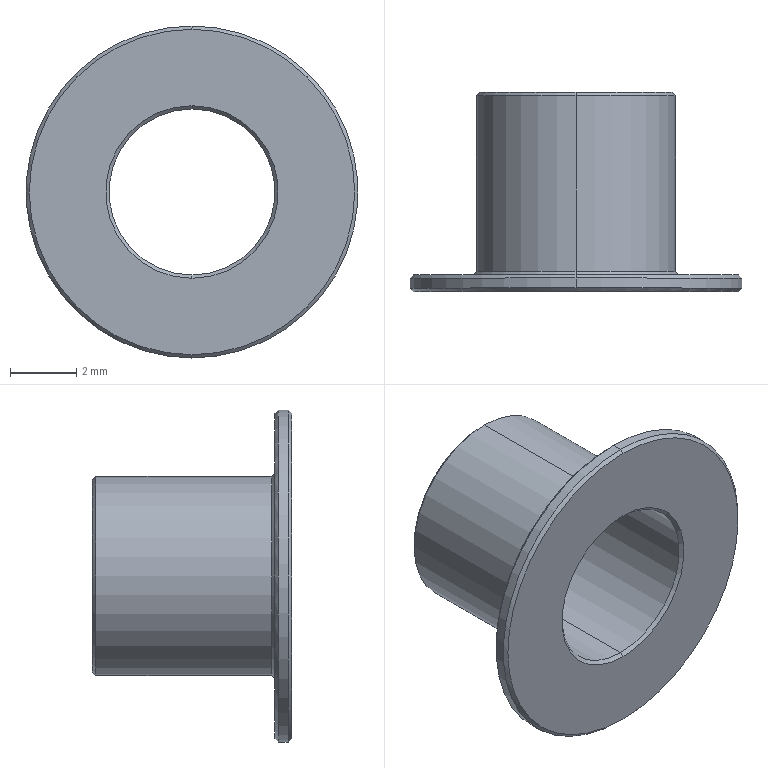Part | SolidWorks | features Chamfer 1, Revolution 1 | 1 solid | 21 faces | box 10 x 6 x 10 mm | volume 76.5 mm3 | cone 12 | cylinder 6 | plane 3 | commonest cylinder face diameters 5 x2 6 x2 10 x2
STEP:
#1=CARTESIAN_POINT('',(0.,6.,2.9));
#2=VERTEX_POINT('',#1);
#3=CARTESIAN_POINT('',(0.,6.,-2.9));
#4=VERTEX_POINT('',#3);
#5=CARTESIAN_POINT('',(0.,6.,0.));
#6=DIRECTION('',(0.,1.,0.));
#7=DIRECTION('',(0.,0.,1.));
#8=AXIS2_PLACEMENT_3D('',#5,#6,#7);
#9=CIRCLE('',#8,2.9);
#10=EDGE_CURVE('',#2,#4,#9,.T.);
#11=ORIENTED_EDGE('',*,*,#10,.F.);
#12=CARTESIAN_POINT('',(0.,5.9,3.));
#13=VERTEX_POINT('',#12);
#14=CARTESIAN_POINT('',(0.,5.9,3.));
#15=DIRECTION('',(0.,-0.7071,0.7071));
#16=VECTOR('',#15,1000.);
#17=LINE('',#14,#16);
#18=EDGE_CURVE('',#2,#13,#17,.T.);
#19=ORIENTED_EDGE('',*,*,#18,.T.);
#20=CARTESIAN_POINT('',(0.,5.9,-3.));
#21=VERTEX_POINT('',#20);
#22=CARTESIAN_POINT('',(0.,5.9,0.));
#23=DIRECTION('',(0.,-1.,0.));
#24=DIRECTION('',(0.,0.,1.));
#25=AXIS2_PLACEMENT_3D('',#22,#23,#24);
#26=CIRCLE('',#25,3.);
#27=EDGE_CURVE('',#21,#13,#26,.T.);
#28=ORIENTED_EDGE('',*,*,#27,.F.);
#29=CARTESIAN_POINT('',(0.,5.9,-3.));
#30=DIRECTION('',(0.,-0.7071,-0.7071));
#31=VECTOR('',#30,1000.);
#32=LINE('',#29,#31);
#33=EDGE_CURVE('',#4,#21,#32,.T.);
#34=ORIENTED_EDGE('',*,*,#33,.F.);
#35=EDGE_LOOP('',(#11,#19,#28,#34));
#36=FACE_OUTER_BOUND('',#35,.T.);
#37=CARTESIAN_POINT('',(0.,5.9,0.));
#38=DIRECTION('',(0.,-1.,0.));
#39=DIRECTION('',(0.,0.,-1.));
#40=AXIS2_PLACEMENT_3D('',#37,#38,#39);
#41=CONICAL_SURFACE('',#40,3.,0.7854);
#42=ADVANCED_FACE('',(#36),#41,.T.);
#43=CARTESIAN_POINT('',(0.,5.9,-2.5));
#44=VERTEX_POINT('',#43);
#45=CARTESIAN_POINT('',(0.,5.9,2.5));
#46=VERTEX_POINT('',#45);
#47=CARTESIAN_POINT('',(0.,5.9,0.));
#48=DIRECTION('',(0.,1.,0.));
#49=DIRECTION('',(0.,0.,1.));
#50=AXIS2_PLACEMENT_3D('',#47,#48,#49);
#51=CIRCLE('',#50,2.5);
#52=EDGE_CURVE('',#44,#46,#51,.T.);
#53=ORIENTED_EDGE('',*,*,#52,.F.);
#54=CARTESIAN_POINT('',(0.,6.,-2.6));
#55=VERTEX_POINT('',#54);
#56=CARTESIAN_POINT('',(0.,6.,-2.6));
#57=DIRECTION('',(0.,0.7071,-0.7071));
#58=VECTOR('',#57,1000.);
#59=LINE('',#56,#58);
#60=EDGE_CURVE('',#44,#55,#59,.T.);
#61=ORIENTED_EDGE('',*,*,#60,.T.);
#62=CARTESIAN_POINT('',(0.,6.,2.6));
#63=VERTEX_POINT('',#62);
#64=CARTESIAN_POINT('',(0.,6.,0.));
#65=DIRECTION('',(0.,-1.,0.));
#66=DIRECTION('',(0.,0.,1.));
#67=AXIS2_PLACEMENT_3D('',#64,#65,#66);
#68=CIRCLE('',#67,2.6);
#69=EDGE_CURVE('',#63,#55,#68,.T.);
#70=ORIENTED_EDGE('',*,*,#69,.F.);
#71=CARTESIAN_POINT('',(0.,6.,2.6));
#72=DIRECTION('',(0.,0.7071,0.7071));
#73=VECTOR('',#72,1000.);
#74=LINE('',#71,#73);
#75=EDGE_CURVE('',#46,#63,#74,.T.);
#76=ORIENTED_EDGE('',*,*,#75,.F.);
#77=EDGE_LOOP('',(#53,#61,#70,#76));
#78=FACE_OUTER_BOUND('',#77,.T.);
#79=CARTESIAN_POINT('',(0.,6.,0.));
#80=DIRECTION('',(0.,1.,0.));
#81=DIRECTION('',(0.,0.,1.));
#82=AXIS2_PLACEMENT_3D('',#79,#80,#81);
#83=CONICAL_SURFACE('',#82,2.6,0.7854);
#84=ADVANCED_FACE('',(#78),#83,.F.);
#85=CARTESIAN_POINT('',(0.,0.5,4.9));
#86=VERTEX_POINT('',#85);
#87=CARTESIAN_POINT('',(0.,0.5,-4.9));
#88=VERTEX_POINT('',#87);
#89=CARTESIAN_POINT('',(0.,0.5,0.));
#90=DIRECTION('',(0.,1.,0.));
#91=DIRECTION('',(0.,0.,1.));
#92=AXIS2_PLACEMENT_3D('',#89,#90,#91);
#93=CIRCLE('',#92,4.9);
#94=EDGE_CURVE('',#86,#88,#93,.T.);
#95=ORIENTED_EDGE('',*,*,#94,.F.);
#96=CARTESIAN_POINT('',(0.,0.4,5.));
#97=VERTEX_POINT('',#96);
#98=CARTESIAN_POINT('',(0.,0.4,5.));
#99=DIRECTION('',(0.,-0.7071,0.7071));
#100=VECTOR('',#99,1000.);
#101=LINE('',#98,#100);
#102=EDGE_CURVE('',#86,#97,#101,.T.);
#103=ORIENTED_EDGE('',*,*,#102,.T.);
#104=CARTESIAN_POINT('',(0.,0.4,-5.));
#105=VERTEX_POINT('',#104);
#106=CARTESIAN_POINT('',(0.,0.4,0.));
#107=DIRECTION('',(0.,-1.,0.));
#108=DIRECTION('',(0.,0.,1.));
#109=AXIS2_PLACEMENT_3D('',#106,#107,#108);
#110=CIRCLE('',#109,5.);
#111=EDGE_CURVE('',#105,#97,#110,.T.);
#112=ORIENTED_EDGE('',*,*,#111,.F.);
#113=CARTESIAN_POINT('',(0.,0.4,-5.));
#114=DIRECTION('',(0.,-0.7071,-0.7071));
#115=VECTOR('',#114,1000.);
#116=LINE('',#113,#115);
#117=EDGE_CURVE('',#88,#105,#116,.T.);
#118=ORIENTED_EDGE('',*,*,#117,.F.);
#119=EDGE_LOOP('',(#95,#103,#112,#118));
#120=FACE_OUTER_BOUND('',#119,.T.);
#121=CARTESIAN_POINT('',(0.,0.4,0.));
#122=DIRECTION('',(0.,-1.,0.));
#123=DIRECTION('',(0.,0.,-1.));
#124=AXIS2_PLACEMENT_3D('',#121,#122,#123);
#125=CONICAL_SURFACE('',#124,5.,0.7854);
#126=ADVANCED_FACE('',(#120),#125,.T.);
#127=CARTESIAN_POINT('',(0.,0.,-4.9));
#128=VERTEX_POINT('',#127);
#129=CARTESIAN_POINT('',(0.,0.,4.9));
#130=VERTEX_POINT('',#129);
#131=CARTESIAN_POINT('',(0.,0.,0.));
#132=DIRECTION('',(0.,-1.,0.));
#133=DIRECTION('',(0.,0.,-1.));
#134=AXIS2_PLACEMENT_3D('',#131,#132,#133);
#135=CIRCLE('',#134,4.9);
#136=EDGE_CURVE('',#128,#130,#135,.T.);
#137=ORIENTED_EDGE('',*,*,#136,.F.);
#138=CARTESIAN_POINT('',(0.,0.1,-5.));
#139=VERTEX_POINT('',#138);
#140=CARTESIAN_POINT('',(0.,0.,-4.9));
#141=DIRECTION('',(0.,0.7071,-0.7071));
#142=VECTOR('',#141,1000.);
#143=LINE('',#140,#142);
#144=EDGE_CURVE('',#128,#139,#143,.T.);
#145=ORIENTED_EDGE('',*,*,#144,.T.);
#146=CARTESIAN_POINT('',(0.,0.1,5.));
#147=VERTEX_POINT('',#146);
#148=CARTESIAN_POINT('',(0.,0.1,0.));
#149=DIRECTION('',(0.,1.,0.));
#150=DIRECTION('',(0.,0.,-1.));
#151=AXIS2_PLACEMENT_3D('',#148,#149,#150);
#152=CIRCLE('',#151,5.);
#153=EDGE_CURVE('',#147,#139,#152,.T.);
#154=ORIENTED_EDGE('',*,*,#153,.F.);
#155=CARTESIAN_POINT('',(0.,0.,4.9));
#156=DIRECTION('',(0.,0.7071,0.7071));
#157=VECTOR('',#156,1000.);
#158=LINE('',#155,#157);
#159=EDGE_CURVE('',#130,#147,#158,.T.);
#160=ORIENTED_EDGE('',*,*,#159,.F.);
#161=EDGE_LOOP('',(#137,#145,#154,#160));
#162=FACE_OUTER_BOUND('',#161,.T.);
#163=CARTESIAN_POINT('',(0.,0.,0.));
#164=DIRECTION('',(0.,1.,0.));
#165=DIRECTION('',(0.,0.,1.));
#166=AXIS2_PLACEMENT_3D('',#163,#164,#165);
#167=CONICAL_SURFACE('',#166,4.9,0.7854);
#168=ADVANCED_FACE('',(#162),#167,.T.);
#169=CARTESIAN_POINT('',(0.,0.1,2.5));
#170=VERTEX_POINT('',#169);
#171=CARTESIAN_POINT('',(0.,0.1,-2.5));
#172=VERTEX_POINT('',#171);
#173=CARTESIAN_POINT('',(0.,0.1,0.));
#174=DIRECTION('',(0.,-1.,0.));
#175=DIRECTION('',(0.,0.,-1.));
#176=AXIS2_PLACEMENT_3D('',#173,#174,#175);
#177=CIRCLE('',#176,2.5);
#178=EDGE_CURVE('',#170,#172,#177,.T.);
#179=ORIENTED_EDGE('',*,*,#178,.F.);
#180=CARTESIAN_POINT('',(0.,0.,2.6));
#181=VERTEX_POINT('',#180);
#182=CARTESIAN_POINT('',(0.,0.1,2.5));
#183=DIRECTION('',(0.,-0.7071,0.7071));
#184=VECTOR('',#183,1000.);
#185=LINE('',#182,#184);
#186=EDGE_CURVE('',#170,#181,#185,.T.);
#187=ORIENTED_EDGE('',*,*,#186,.T.);
#188=CARTESIAN_POINT('',(0.,0.,-2.6));
#189=VERTEX_POINT('',#188);
#190=CARTESIAN_POINT('',(0.,0.,0.));
#191=DIRECTION('',(0.,1.,0.));
#192=DIRECTION('',(0.,0.,-1.));
#193=AXIS2_PLACEMENT_3D('',#190,#191,#192);
#194=CIRCLE('',#193,2.6);
#195=EDGE_CURVE('',#189,#181,#194,.T.);
#196=ORIENTED_EDGE('',*,*,#195,.F.);
#197=CARTESIAN_POINT('',(0.,0.1,-2.5));
#198=DIRECTION('',(0.,-0.7071,-0.7071));
#199=VECTOR('',#198,1000.);
#200=LINE('',#197,#199);
#201=EDGE_CURVE('',#172,#189,#200,.T.);
#202=ORIENTED_EDGE('',*,*,#201,.F.);
#203=EDGE_LOOP('',(#179,#187,#196,#202));
#204=FACE_OUTER_BOUND('',#203,.T.);
#205=CARTESIAN_POINT('',(0.,0.1,0.));
#206=DIRECTION('',(0.,-1.,0.));
#207=DIRECTION('',(0.,0.,-1.));
#208=AXIS2_PLACEMENT_3D('',#205,#206,#207);
#209=CONICAL_SURFACE('',#208,2.5,0.7854);
#210=ADVANCED_FACE('',(#204),#209,.F.);
#211=CARTESIAN_POINT('',(0.,0.6,3.));
#212=VERTEX_POINT('',#211);
#213=CARTESIAN_POINT('',(0.,0.6,-3.));
#214=VERTEX_POINT('',#213);
#215=CARTESIAN_POINT('',(0.,0.6,0.));
#216=DIRECTION('',(0.,1.,0.));
#217=DIRECTION('',(0.,0.,1.));
#218=AXIS2_PLACEMENT_3D('',#215,#216,#217);
#219=CIRCLE('',#218,3.);
#220=EDGE_CURVE('',#212,#214,#219,.T.);
#221=ORIENTED_EDGE('',*,*,#220,.F.);
#222=CARTESIAN_POINT('',(0.,0.5,3.1));
#223=VERTEX_POINT('',#222);
#224=CARTESIAN_POINT('',(0.,0.5,3.1));
#225=DIRECTION('',(0.,-0.7071,0.7071));
#226=VECTOR('',#225,1000.);
#227=LINE('',#224,#226);
#228=EDGE_CURVE('',#212,#223,#227,.T.);
#229=ORIENTED_EDGE('',*,*,#228,.T.);
#230=CARTESIAN_POINT('',(0.,0.5,-3.1));
#231=VERTEX_POINT('',#230);
#232=CARTESIAN_POINT('',(0.,0.5,0.));
#233=DIRECTION('',(0.,-1.,0.));
#234=DIRECTION('',(0.,0.,1.));
#235=AXIS2_PLACEMENT_3D('',#232,#233,#234);
#236=CIRCLE('',#235,3.1);
#237=EDGE_CURVE('',#231,#223,#236,.T.);
#238=ORIENTED_EDGE('',*,*,#237,.F.);
#239=CARTESIAN_POINT('',(0.,0.5,-3.1));
#240=DIRECTION('',(0.,-0.7071,-0.7071));
#241=VECTOR('',#240,1000.);
#242=LINE('',#239,#241);
#243=EDGE_CURVE('',#214,#231,#242,.T.);
#244=ORIENTED_EDGE('',*,*,#243,.F.);
#245=EDGE_LOOP('',(#221,#229,#238,#244));
#246=FACE_OUTER_BOUND('',#245,.T.);
#247=CARTESIAN_POINT('',(0.,0.5,0.));
#248=DIRECTION('',(0.,-1.,0.));
#249=DIRECTION('',(0.,0.,-1.));
#250=AXIS2_PLACEMENT_3D('',#247,#248,#249);
#251=CONICAL_SURFACE('',#250,3.1,0.7854);
#252=ADVANCED_FACE('',(#246),#251,.T.);
#253=ORIENTED_EDGE('',*,*,#27,.T.);
#254=CARTESIAN_POINT('',(0.,0.,3.));
#255=DIRECTION('',(0.,-1.,0.));
#256=VECTOR('',#255,1000.);
#257=LINE('',#254,#256);
#258=EDGE_CURVE('',#13,#212,#257,.T.);
#259=ORIENTED_EDGE('',*,*,#258,.T.);
#260=ORIENTED_EDGE('',*,*,#220,.T.);
#261=CARTESIAN_POINT('',(0.,0.,-3.));
#262=DIRECTION('',(0.,-1.,0.));
#263=VECTOR('',#262,1000.);
#264=LINE('',#261,#263);
#265=EDGE_CURVE('',#21,#214,#264,.T.);
#266=ORIENTED_EDGE('',*,*,#265,.F.);
#267=EDGE_LOOP('',(#253,#259,#260,#266));
#268=FACE_OUTER_BOUND('',#267,.T.);
#269=CARTESIAN_POINT('',(0.,0.,0.));
#270=DIRECTION('',(0.,-1.,0.));
#271=DIRECTION('',(0.,0.,-1.));
#272=AXIS2_PLACEMENT_3D('',#269,#270,#271);
#273=CYLINDRICAL_SURFACE('',#272,3.);
#274=ADVANCED_FACE('',(#268),#273,.T.);
#275=ORIENTED_EDGE('',*,*,#111,.T.);
#276=CARTESIAN_POINT('',(0.,0.,5.));
#277=DIRECTION('',(0.,-1.,0.));
#278=VECTOR('',#277,1000.);
#279=LINE('',#276,#278);
#280=EDGE_CURVE('',#97,#147,#279,.T.);
#281=ORIENTED_EDGE('',*,*,#280,.T.);
#282=ORIENTED_EDGE('',*,*,#153,.T.);
#283=CARTESIAN_POINT('',(0.,0.,-5.));
#284=DIRECTION('',(0.,-1.,0.));
#285=VECTOR('',#284,1000.);
#286=LINE('',#283,#285);
#287=EDGE_CURVE('',#105,#139,#286,.T.);
#288=ORIENTED_EDGE('',*,*,#287,.F.);
#289=EDGE_LOOP('',(#275,#281,#282,#288));
#290=FACE_OUTER_BOUND('',#289,.T.);
#291=CARTESIAN_POINT('',(0.,0.,0.));
#292=DIRECTION('',(0.,-1.,0.));
#293=DIRECTION('',(0.,0.,-1.));
#294=AXIS2_PLACEMENT_3D('',#291,#292,#293);
#295=CYLINDRICAL_SURFACE('',#294,5.);
#296=ADVANCED_FACE('',(#290),#295,.T.);
#297=ORIENTED_EDGE('',*,*,#52,.T.);
#298=CARTESIAN_POINT('',(0.,0.,2.5));
#299=DIRECTION('',(0.,-1.,0.));
#300=VECTOR('',#299,1000.);
#301=LINE('',#298,#300);
#302=EDGE_CURVE('',#46,#170,#301,.T.);
#303=ORIENTED_EDGE('',*,*,#302,.T.);
#304=ORIENTED_EDGE('',*,*,#178,.T.);
#305=CARTESIAN_POINT('',(0.,0.,-2.5));
#306=DIRECTION('',(0.,-1.,0.));
#307=VECTOR('',#306,1000.);
#308=LINE('',#305,#307);
#309=EDGE_CURVE('',#44,#172,#308,.T.);
#310=ORIENTED_EDGE('',*,*,#309,.F.);
#311=EDGE_LOOP('',(#297,#303,#304,#310));
#312=FACE_OUTER_BOUND('',#311,.T.);
#313=CARTESIAN_POINT('',(0.,0.,0.));
#314=DIRECTION('',(0.,-1.,0.));
#315=DIRECTION('',(0.,0.,-1.));
#316=AXIS2_PLACEMENT_3D('',#313,#314,#315);
#317=CYLINDRICAL_SURFACE('',#316,2.5);
#318=ADVANCED_FACE('',(#312),#317,.F.);
#319=ORIENTED_EDGE('',*,*,#302,.F.);
#320=CARTESIAN_POINT('',(0.,5.9,0.));
#321=DIRECTION('',(0.,1.,0.));
#322=DIRECTION('',(0.,0.,1.));
#323=AXIS2_PLACEMENT_3D('',#320,#321,#322);
#324=CIRCLE('',#323,2.5);
#325=EDGE_CURVE('',#46,#44,#324,.T.);
#326=ORIENTED_EDGE('',*,*,#325,.T.);
#327=ORIENTED_EDGE('',*,*,#309,.T.);
#328=CARTESIAN_POINT('',(0.,0.1,0.));
#329=DIRECTION('',(0.,-1.,0.));
#330=DIRECTION('',(0.,0.,-1.));
#331=AXIS2_PLACEMENT_3D('',#328,#329,#330);
#332=CIRCLE('',#331,2.5);
#333=EDGE_CURVE('',#172,#170,#332,.T.);
#334=ORIENTED_EDGE('',*,*,#333,.T.);
#335=EDGE_LOOP('',(#319,#326,#327,#334));
#336=FACE_OUTER_BOUND('',#335,.T.);
#337=CARTESIAN_POINT('',(0.,0.,0.));
#338=DIRECTION('',(0.,-1.,0.));
#339=DIRECTION('',(0.,0.,-1.));
#340=AXIS2_PLACEMENT_3D('',#337,#338,#339);
#341=CYLINDRICAL_SURFACE('',#340,2.5);
#342=ADVANCED_FACE('',(#336),#341,.F.);
#343=ORIENTED_EDGE('',*,*,#195,.T.);
#344=CARTESIAN_POINT('',(0.,0.,0.));
#345=DIRECTION('',(0.,1.,0.));
#346=DIRECTION('',(0.,0.,-1.));
#347=AXIS2_PLACEMENT_3D('',#344,#345,#346);
#348=CIRCLE('',#347,2.6);
#349=EDGE_CURVE('',#181,#189,#348,.T.);
#350=ORIENTED_EDGE('',*,*,#349,.T.);
#351=EDGE_LOOP('',(#343,#350));
#352=FACE_BOUND('',#351,.T.);
#353=CARTESIAN_POINT('',(0.,0.,0.));
#354=DIRECTION('',(0.,-1.,0.));
#355=DIRECTION('',(0.,0.,-1.));
#356=AXIS2_PLACEMENT_3D('',#353,#354,#355);
#357=CIRCLE('',#356,4.9);
#358=EDGE_CURVE('',#130,#128,#357,.T.);
#359=ORIENTED_EDGE('',*,*,#358,.T.);
#360=ORIENTED_EDGE('',*,*,#136,.T.);
#361=EDGE_LOOP('',(#359,#360));
#362=FACE_OUTER_BOUND('',#361,.T.);
#363=CARTESIAN_POINT('',(2.5,0.,0.));
#364=DIRECTION('',(0.,-1.,0.));
#365=DIRECTION('',(0.,0.,-1.));
#366=AXIS2_PLACEMENT_3D('',#363,#364,#365);
#367=PLANE('',#366);
#368=ADVANCED_FACE('',(#352,#362),#367,.T.);
#369=ORIENTED_EDGE('',*,*,#280,.F.);
#370=CARTESIAN_POINT('',(0.,0.4,0.));
#371=DIRECTION('',(0.,-1.,0.));
#372=DIRECTION('',(0.,0.,1.));
#373=AXIS2_PLACEMENT_3D('',#370,#371,#372);
#374=CIRCLE('',#373,5.);
#375=EDGE_CURVE('',#97,#105,#374,.T.);
#376=ORIENTED_EDGE('',*,*,#375,.T.);
#377=ORIENTED_EDGE('',*,*,#287,.T.);
#378=CARTESIAN_POINT('',(0.,0.1,0.));
#379=DIRECTION('',(0.,1.,0.));
#380=DIRECTION('',(0.,0.,-1.));
#381=AXIS2_PLACEMENT_3D('',#378,#379,#380);
#382=CIRCLE('',#381,5.);
#383=EDGE_CURVE('',#139,#147,#382,.T.);
#384=ORIENTED_EDGE('',*,*,#383,.T.);
#385=EDGE_LOOP('',(#369,#376,#377,#384));
#386=FACE_OUTER_BOUND('',#385,.T.);
#387=CARTESIAN_POINT('',(0.,0.,0.));
#388=DIRECTION('',(0.,-1.,0.));
#389=DIRECTION('',(0.,0.,-1.));
#390=AXIS2_PLACEMENT_3D('',#387,#388,#389);
#391=CYLINDRICAL_SURFACE('',#390,5.);
#392=ADVANCED_FACE('',(#386),#391,.T.);
#393=ORIENTED_EDGE('',*,*,#237,.T.);
#394=CARTESIAN_POINT('',(0.,0.5,0.));
#395=DIRECTION('',(0.,-1.,0.));
#396=DIRECTION('',(0.,0.,1.));
#397=AXIS2_PLACEMENT_3D('',#394,#395,#396);
#398=CIRCLE('',#397,3.1);
#399=EDGE_CURVE('',#223,#231,#398,.T.);
#400=ORIENTED_EDGE('',*,*,#399,.T.);
#401=EDGE_LOOP('',(#393,#400));
#402=FACE_BOUND('',#401,.T.);
#403=CARTESIAN_POINT('',(0.,0.5,0.));
#404=DIRECTION('',(0.,1.,0.));
#405=DIRECTION('',(0.,0.,1.));
#406=AXIS2_PLACEMENT_3D('',#403,#404,#405);
#407=CIRCLE('',#406,4.9);
#408=EDGE_CURVE('',#88,#86,#407,.T.);
#409=ORIENTED_EDGE('',*,*,#408,.T.);
#410=ORIENTED_EDGE('',*,*,#94,.T.);
#411=EDGE_LOOP('',(#409,#410));
#412=FACE_OUTER_BOUND('',#411,.T.);
#413=CARTESIAN_POINT('',(5.,0.5,0.));
#414=DIRECTION('',(0.,1.,0.));
#415=DIRECTION('',(0.,0.,1.));
#416=AXIS2_PLACEMENT_3D('',#413,#414,#415);
#417=PLANE('',#416);
#418=ADVANCED_FACE('',(#402,#412),#417,.T.);
#419=ORIENTED_EDGE('',*,*,#258,.F.);
#420=CARTESIAN_POINT('',(0.,5.9,0.));
#421=DIRECTION('',(0.,-1.,0.));
#422=DIRECTION('',(0.,0.,1.));
#423=AXIS2_PLACEMENT_3D('',#420,#421,#422);
#424=CIRCLE('',#423,3.);
#425=EDGE_CURVE('',#13,#21,#424,.T.);
#426=ORIENTED_EDGE('',*,*,#425,.T.);
#427=ORIENTED_EDGE('',*,*,#265,.T.);
#428=CARTESIAN_POINT('',(0.,0.6,0.));
#429=DIRECTION('',(0.,1.,0.));
#430=DIRECTION('',(0.,0.,1.));
#431=AXIS2_PLACEMENT_3D('',#428,#429,#430);
#432=CIRCLE('',#431,3.);
#433=EDGE_CURVE('',#214,#212,#432,.T.);
#434=ORIENTED_EDGE('',*,*,#433,.T.);
#435=EDGE_LOOP('',(#419,#426,#427,#434));
#436=FACE_OUTER_BOUND('',#435,.T.);
#437=CARTESIAN_POINT('',(0.,0.,0.));
#438=DIRECTION('',(0.,-1.,0.));
#439=DIRECTION('',(0.,0.,-1.));
#440=AXIS2_PLACEMENT_3D('',#437,#438,#439);
#441=CYLINDRICAL_SURFACE('',#440,3.);
#442=ADVANCED_FACE('',(#436),#441,.T.);
#443=ORIENTED_EDGE('',*,*,#69,.T.);
#444=CARTESIAN_POINT('',(0.,6.,0.));
#445=DIRECTION('',(0.,-1.,0.));
#446=DIRECTION('',(0.,0.,1.));
#447=AXIS2_PLACEMENT_3D('',#444,#445,#446);
#448=CIRCLE('',#447,2.6);
#449=EDGE_CURVE('',#55,#63,#448,.T.);
#450=ORIENTED_EDGE('',*,*,#449,.T.);
#451=EDGE_LOOP('',(#443,#450));
#452=FACE_BOUND('',#451,.T.);
#453=CARTESIAN_POINT('',(0.,6.,0.));
#454=DIRECTION('',(0.,1.,0.));
#455=DIRECTION('',(0.,0.,1.));
#456=AXIS2_PLACEMENT_3D('',#453,#454,#455);
#457=CIRCLE('',#456,2.9);
#458=EDGE_CURVE('',#4,#2,#457,.T.);
#459=ORIENTED_EDGE('',*,*,#458,.T.);
#460=ORIENTED_EDGE('',*,*,#10,.T.);
#461=EDGE_LOOP('',(#459,#460));
#462=FACE_OUTER_BOUND('',#461,.T.);
#463=CARTESIAN_POINT('',(3.,6.,0.));
#464=DIRECTION('',(0.,1.,0.));
#465=DIRECTION('',(0.,0.,1.));
#466=AXIS2_PLACEMENT_3D('',#463,#464,#465);
#467=PLANE('',#466);
#468=ADVANCED_FACE('',(#452,#462),#467,.T.);
#469=ORIENTED_EDGE('',*,*,#228,.F.);
#470=ORIENTED_EDGE('',*,*,#433,.F.);
#471=ORIENTED_EDGE('',*,*,#243,.T.);
#472=ORIENTED_EDGE('',*,*,#399,.F.);
#473=EDGE_LOOP('',(#469,#470,#471,#472));
#474=FACE_OUTER_BOUND('',#473,.T.);
#475=CARTESIAN_POINT('',(0.,0.5,0.));
#476=DIRECTION('',(0.,-1.,0.));
#477=DIRECTION('',(0.,0.,-1.));
#478=AXIS2_PLACEMENT_3D('',#475,#476,#477);
#479=CONICAL_SURFACE('',#478,3.1,0.7854);
#480=ADVANCED_FACE('',(#474),#479,.T.);
#481=ORIENTED_EDGE('',*,*,#186,.F.);
#482=ORIENTED_EDGE('',*,*,#333,.F.);
#483=ORIENTED_EDGE('',*,*,#201,.T.);
#484=ORIENTED_EDGE('',*,*,#349,.F.);
#485=EDGE_LOOP('',(#481,#482,#483,#484));
#486=FACE_OUTER_BOUND('',#485,.T.);
#487=CARTESIAN_POINT('',(0.,0.1,0.));
#488=DIRECTION('',(0.,-1.,0.));
#489=DIRECTION('',(0.,0.,-1.));
#490=AXIS2_PLACEMENT_3D('',#487,#488,#489);
#491=CONICAL_SURFACE('',#490,2.5,0.7854);
#492=ADVANCED_FACE('',(#486),#491,.F.);
#493=ORIENTED_EDGE('',*,*,#144,.F.);
#494=ORIENTED_EDGE('',*,*,#358,.F.);
#495=ORIENTED_EDGE('',*,*,#159,.T.);
#496=ORIENTED_EDGE('',*,*,#383,.F.);
#497=EDGE_LOOP('',(#493,#494,#495,#496));
#498=FACE_OUTER_BOUND('',#497,.T.);
#499=CARTESIAN_POINT('',(0.,0.,0.));
#500=DIRECTION('',(0.,1.,0.));
#501=DIRECTION('',(0.,0.,1.));
#502=AXIS2_PLACEMENT_3D('',#499,#500,#501);
#503=CONICAL_SURFACE('',#502,4.9,0.7854);
#504=ADVANCED_FACE('',(#498),#503,.T.);
#505=ORIENTED_EDGE('',*,*,#102,.F.);
#506=ORIENTED_EDGE('',*,*,#408,.F.);
#507=ORIENTED_EDGE('',*,*,#117,.T.);
#508=ORIENTED_EDGE('',*,*,#375,.F.);
#509=EDGE_LOOP('',(#505,#506,#507,#508));
#510=FACE_OUTER_BOUND('',#509,.T.);
#511=CARTESIAN_POINT('',(0.,0.4,0.));
#512=DIRECTION('',(0.,-1.,0.));
#513=DIRECTION('',(0.,0.,-1.));
#514=AXIS2_PLACEMENT_3D('',#511,#512,#513);
#515=CONICAL_SURFACE('',#514,5.,0.7854);
#516=ADVANCED_FACE('',(#510),#515,.T.);
#517=ORIENTED_EDGE('',*,*,#60,.F.);
#518=ORIENTED_EDGE('',*,*,#325,.F.);
#519=ORIENTED_EDGE('',*,*,#75,.T.);
#520=ORIENTED_EDGE('',*,*,#449,.F.);
#521=EDGE_LOOP('',(#517,#518,#519,#520));
#522=FACE_OUTER_BOUND('',#521,.T.);
#523=CARTESIAN_POINT('',(0.,6.,0.));
#524=DIRECTION('',(0.,1.,0.));
#525=DIRECTION('',(0.,0.,1.));
#526=AXIS2_PLACEMENT_3D('',#523,#524,#525);
#527=CONICAL_SURFACE('',#526,2.6,0.7854);
#528=ADVANCED_FACE('',(#522),#527,.F.);
#529=ORIENTED_EDGE('',*,*,#18,.F.);
#530=ORIENTED_EDGE('',*,*,#458,.F.);
#531=ORIENTED_EDGE('',*,*,#33,.T.);
#532=ORIENTED_EDGE('',*,*,#425,.F.);
#533=EDGE_LOOP('',(#529,#530,#531,#532));
#534=FACE_OUTER_BOUND('',#533,.T.);
#535=CARTESIAN_POINT('',(0.,5.9,0.));
#536=DIRECTION('',(0.,-1.,0.));
#537=DIRECTION('',(0.,0.,-1.));
#538=AXIS2_PLACEMENT_3D('',#535,#536,#537);
#539=CONICAL_SURFACE('',#538,3.,0.7854);
#540=ADVANCED_FACE('',(#534),#539,.T.);
#541=CLOSED_SHELL('',(#42,#84,#126,#168,#210,#252,#274,#296,#318,#342,#368,#392,#418,#442,#468,#480,#492,#504,#516,#528,#540));
#542=MANIFOLD_SOLID_BREP('',#541);
#543=CARTESIAN_POINT('',(0.,0.,0.));
#544=DIRECTION('',(0.,0.,1.));
#545=DIRECTION('',(1.,0.,0.));
#546=AXIS2_PLACEMENT_3D('',#543,#544,#545);
#547=(LENGTH_UNIT()NAMED_UNIT(*)SI_UNIT(.MILLI.,.METRE.));
#548=UNCERTAINTY_MEASURE_WITH_UNIT(LENGTH_MEASURE(0.00001),#547,'','');
#549=(NAMED_UNIT(*)PLANE_ANGLE_UNIT()SI_UNIT($,.RADIAN.));
#550=(NAMED_UNIT(*)SI_UNIT($,.STERADIAN.)SOLID_ANGLE_UNIT());
#551=(GEOMETRIC_REPRESENTATION_CONTEXT(3)GLOBAL_UNCERTAINTY_ASSIGNED_CONTEXT((#548))GLOBAL_UNIT_ASSIGNED_CONTEXT((#547,#549,#550))REPRESENTATION_CONTEXT('',''));
#552=ADVANCED_BREP_SHAPE_REPRESENTATION('',(#542,#546),#551);